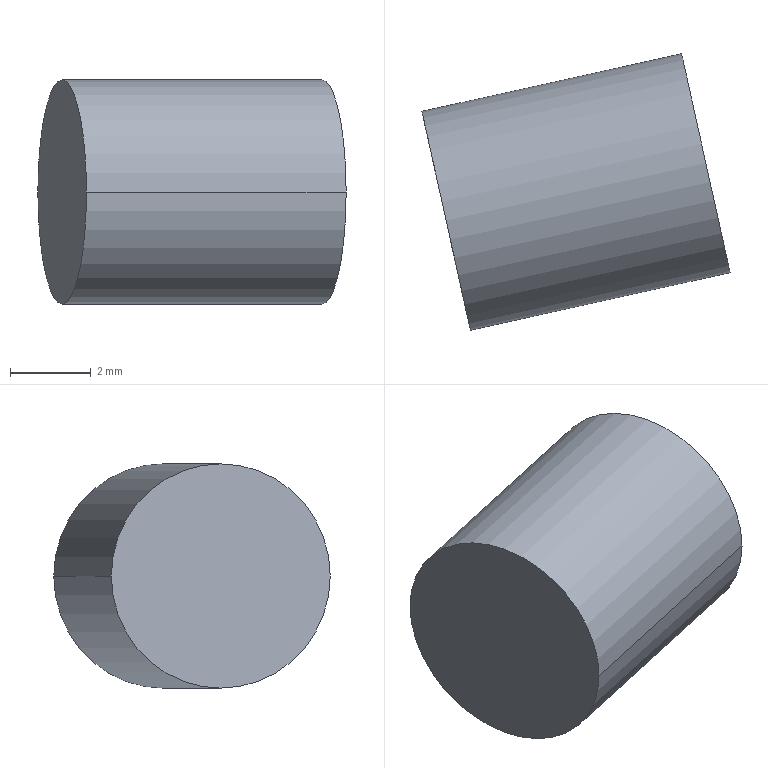Part | NX | features BREP 1 | 1 solid | 4 faces | box 7.648 x 6.86 x 5.563 mm | volume 160.419 mm3 | plane 2 | cylinder 2 | commonest cylinder face diameters 5.563 x2
STEP:
#1=CARTESIAN_POINT('',(8.676,13.165,0.));
#2=VERTEX_POINT('',#1);
#3=CARTESIAN_POINT('',(7.472,18.596,0.));
#4=VERTEX_POINT('',#3);
#5=CARTESIAN_POINT('',(8.074,15.88,0.));
#6=DIRECTION('',(0.9763,0.2164,0.));
#7=DIRECTION('',(0.2164,-0.9763,0.));
#8=AXIS2_PLACEMENT_3D('',#5,#6,#7);
#9=CIRCLE('',#8,2.782);
#10=EDGE_CURVE('',#2,#4,#9,.T.);
#11=ORIENTED_EDGE('',*,*,#10,.T.);
#12=CARTESIAN_POINT('',(8.074,15.88,0.));
#13=DIRECTION('',(0.9763,0.2164,0.));
#14=DIRECTION('',(-0.2164,0.9763,0.));
#15=AXIS2_PLACEMENT_3D('',#12,#13,#14);
#16=CIRCLE('',#15,2.782);
#17=EDGE_CURVE('',#4,#2,#16,.T.);
#18=ORIENTED_EDGE('',*,*,#17,.T.);
#19=EDGE_LOOP('',(#11,#18));
#20=FACE_BOUND('',#19,.T.);
#21=CARTESIAN_POINT('',(8.074,15.88,0.));
#22=DIRECTION('',(0.9763,0.2164,0.));
#23=DIRECTION('',(0.,0.,-1.));
#24=AXIS2_PLACEMENT_3D('',#21,#22,#23);
#25=PLANE('',#24);
#26=ADVANCED_FACE('',(#20),#25,.T.);
#27=CARTESIAN_POINT('',(1.028,17.167,0.));
#28=VERTEX_POINT('',#27);
#29=CARTESIAN_POINT('',(1.028,17.167,0.));
#30=DIRECTION('',(0.9763,0.2164,0.));
#31=VECTOR('',#30,1000.);
#32=LINE('',#29,#31);
#33=EDGE_CURVE('',#28,#4,#32,.T.);
#34=ORIENTED_EDGE('',*,*,#33,.F.);
#35=CARTESIAN_POINT('',(2.232,11.736,0.));
#36=VERTEX_POINT('',#35);
#37=CARTESIAN_POINT('',(1.63,14.452,0.));
#38=DIRECTION('',(-0.9763,-0.2164,0.));
#39=DIRECTION('',(0.2164,-0.9763,0.));
#40=AXIS2_PLACEMENT_3D('',#37,#38,#39);
#41=CIRCLE('',#40,2.782);
#42=EDGE_CURVE('',#36,#28,#41,.T.);
#43=ORIENTED_EDGE('',*,*,#42,.F.);
#44=CARTESIAN_POINT('',(2.232,11.736,0.));
#45=DIRECTION('',(0.9763,0.2164,0.));
#46=VECTOR('',#45,1000.);
#47=LINE('',#44,#46);
#48=EDGE_CURVE('',#36,#2,#47,.T.);
#49=ORIENTED_EDGE('',*,*,#48,.T.);
#50=ORIENTED_EDGE('',*,*,#17,.F.);
#51=EDGE_LOOP('',(#34,#43,#49,#50));
#52=FACE_BOUND('',#51,.T.);
#53=CARTESIAN_POINT('',(1.63,14.452,0.));
#54=DIRECTION('',(-0.9763,-0.2164,0.));
#55=DIRECTION('',(0.2164,-0.9763,0.));
#56=AXIS2_PLACEMENT_3D('',#53,#54,#55);
#57=CYLINDRICAL_SURFACE('',#56,2.782);
#58=ADVANCED_FACE('',(#52),#57,.T.);
#59=ORIENTED_EDGE('',*,*,#10,.F.);
#60=ORIENTED_EDGE('',*,*,#48,.F.);
#61=CARTESIAN_POINT('',(1.63,14.452,0.));
#62=DIRECTION('',(-0.9763,-0.2164,0.));
#63=DIRECTION('',(-0.2164,0.9763,0.));
#64=AXIS2_PLACEMENT_3D('',#61,#62,#63);
#65=CIRCLE('',#64,2.782);
#66=EDGE_CURVE('',#28,#36,#65,.T.);
#67=ORIENTED_EDGE('',*,*,#66,.F.);
#68=ORIENTED_EDGE('',*,*,#33,.T.);
#69=EDGE_LOOP('',(#59,#60,#67,#68));
#70=FACE_BOUND('',#69,.T.);
#71=CARTESIAN_POINT('',(1.63,14.452,0.));
#72=DIRECTION('',(-0.9763,-0.2164,0.));
#73=DIRECTION('',(0.2164,-0.9763,0.));
#74=AXIS2_PLACEMENT_3D('',#71,#72,#73);
#75=CYLINDRICAL_SURFACE('',#74,2.782);
#76=ADVANCED_FACE('',(#70),#75,.T.);
#77=ORIENTED_EDGE('',*,*,#66,.T.);
#78=ORIENTED_EDGE('',*,*,#42,.T.);
#79=EDGE_LOOP('',(#77,#78));
#80=FACE_BOUND('',#79,.T.);
#81=CARTESIAN_POINT('',(2.232,11.736,0.));
#82=DIRECTION('',(-0.9763,-0.2164,0.));
#83=DIRECTION('',(-0.2164,0.9763,0.));
#84=AXIS2_PLACEMENT_3D('',#81,#82,#83);
#85=PLANE('',#84);
#86=ADVANCED_FACE('',(#80),#85,.T.);
#87=CLOSED_SHELL('',(#26,#58,#76,#86));
#88=MANIFOLD_SOLID_BREP('',#87);
#89=(LENGTH_UNIT()NAMED_UNIT(*)SI_UNIT(.MILLI.,.METRE.));
#90=UNCERTAINTY_MEASURE_WITH_UNIT(LENGTH_MEASURE(0.00001),#89,'','');
#91=(NAMED_UNIT(*)PLANE_ANGLE_UNIT()SI_UNIT($,.RADIAN.));
#92=(NAMED_UNIT(*)SI_UNIT($,.STERADIAN.)SOLID_ANGLE_UNIT());
#93=(GEOMETRIC_REPRESENTATION_CONTEXT(3)GLOBAL_UNCERTAINTY_ASSIGNED_CONTEXT((#90))GLOBAL_UNIT_ASSIGNED_CONTEXT((#89,#91,#92))REPRESENTATION_CONTEXT('',''));
#94=ADVANCED_BREP_SHAPE_REPRESENTATION('',(#88),#93);